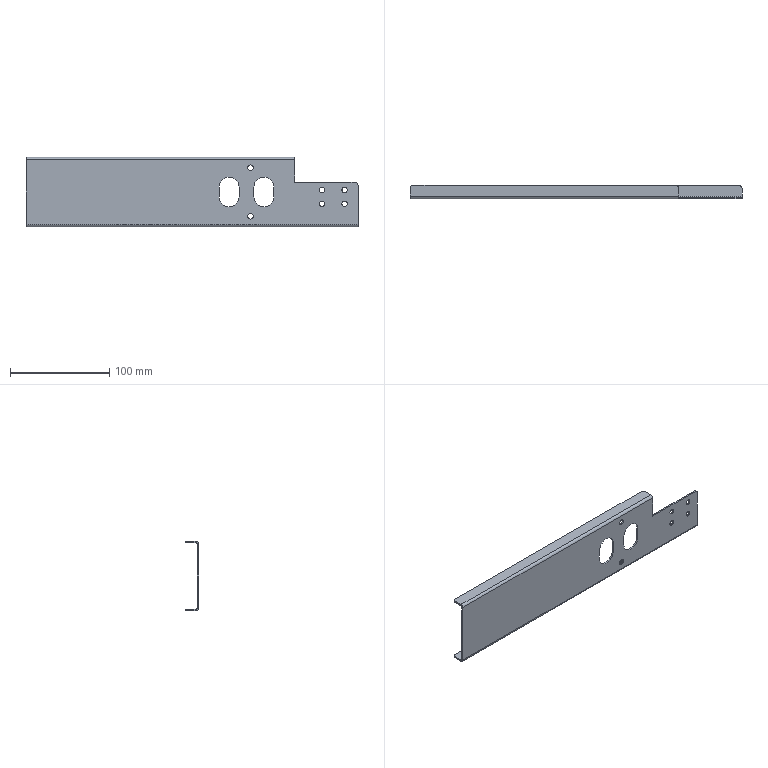Part | SolidWorks | features HoleWzd 3, Cut 1, Fillet 1, FlatPattern 1, ICE 1, LPattern 1, SMBaseFlange 1, SheetMetal 1 | 1 solid | 57 faces | box 335 x 13.5 x 70 mm | volume 41123 mm3 | cylinder 33 | plane 24 | commonest cylinder face diameters 5.5 x18 20 x6 6 x5 2 x2 5 x2